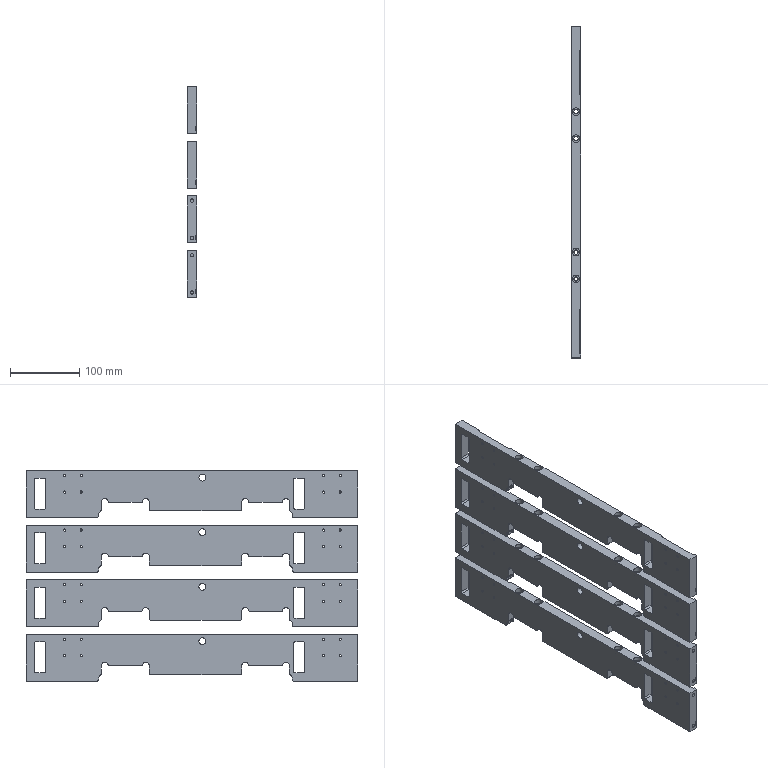Part | 4 solids | 348 faces | box 14 x 480 x 305 mm | volume 1380397 mm3 | cylinder 196 | plane 152 | commonest cylinder face diameters 4 x48 3.2 x32 10 x28 6.5 x16 9.9 x16 10.1 x16